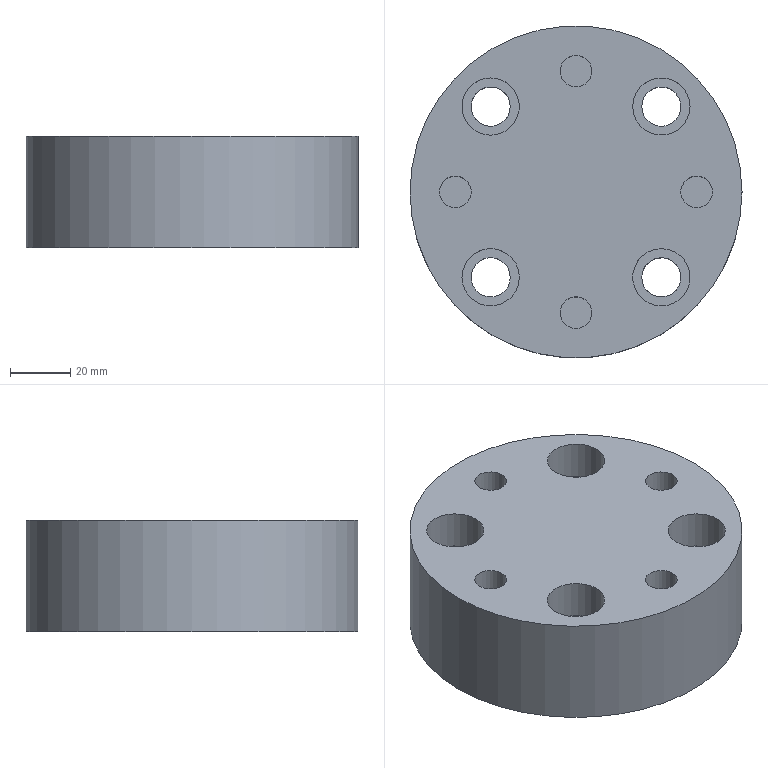NC program | NX | posted with a generic post | part box 110 x 110 x 37 mm
Whole program:
N10 G17 G21 G94 G90
(DRILLING , TOOL : ZXZ)
N12 T01 M6
N14 G54
N16 G17 G0 G90 X0. Y40. S3500 M3
N18 G43 Z30. H1
N20 G94 G81 G98 Z-1. F250. R3.
N22 X-28.284 Y28.284
N24 X-40. Y0.
N26 X-28.284 Y-28.284
N28 X0. Y-40.
N30 X28.284 Y-28.284
N32 X40. Y0.
N34 X28.284 Y28.284
N36 G80
N38 G0 X28.284 Y28.284 Z30.
N40 M5
(DRILLING_COPY , TOOL : 10.5ZT)
N42 T02 M6
N44 G54
N46 G17 G0 G90 X0. Y40. S1200 M3
N48 G43 Z30. H2
N50 G94 G83 G98 Z-28.155 F150. Q3. R3.
N52 X40. Y0.
N54 X0. Y-40.
N56 X-40. Y0.
N58 G80
N60 G0 X-40. Y0. Z30.
N62 M5
(DRILLING_COPY_COPY , TOOL : 13.0ZT)
N64 T03 M6
N66 G54
N68 G17 G0 G90 X-28.284 Y28.284 S500 M3
N70 G43 Z30. H3
N72 G94 G83 G98 Z-41.406 F150. Q3. R3.
N74 X28.284
N76 Y-28.284
N78 X-28.284
N80 G80
N82 G0 X-28.284 Y-28.284 Z30.
N84 M5
(HOLE_MILLING , TOOL : D10)
N86 T10 M6
N88 G54
N90 G17 G0 G90 X-28.284 Y28.284 S3000 M3
N92 G43 Z30. H10
N94 Z0.5
N96 G94 G3 X-26.034 Y26.034 R2.25 F2200.
N98 X-23.784 Y28.284 R2.25
N100 X-23.784 Y28.284 Z0.28 I-4.5 J0.
N102 X-23.784 Y28.284 Z0.06 I-4.5 J0.
N104 X-23.784 Y28.284 Z-0.16 I-4.5 J0.
N106 X-23.784 Y28.284 Z-0.38 I-4.5 J0.
N108 X-23.784 Y28.284 Z-0.6 I-4.5 J0.
N110 X-23.784 Y28.284 Z-0.82 I-4.5 J0.
N112 X-23.784 Y28.284 Z-1.04 I-4.5 J0.
N114 X-23.784 Y28.284 Z-1.26 I-4.5 J0.
N116 X-23.784 Y28.284 Z-1.48 I-4.5 J0.
N118 X-23.784 Y28.284 Z-1.7 I-4.5 J0.
N120 X-23.784 Y28.284 Z-1.92 I-4.5 J0.
N122 X-23.784 Y28.284 Z-2.14 I-4.5 J0.
N124 X-23.784 Y28.284 Z-2.36 I-4.5 J0.
N126 X-23.784 Y28.284 Z-2.58 I-4.5 J0.
N128 X-23.784 Y28.284 Z-2.8 I-4.5 J0.
N130 X-23.784 Y28.284 Z-3.02 I-4.5 J0.
N132 X-23.784 Y28.284 Z-3.24 I-4.5 J0.
N134 X-23.784 Y28.284 Z-3.46 I-4.5 J0.
N136 X-23.784 Y28.284 Z-3.68 I-4.5 J0.
N138 X-23.784 Y28.284 Z-3.9 I-4.5 J0.
N140 X-23.784 Y28.284 Z-4.12 I-4.5 J0.
N142 X-23.784 Y28.284 Z-4.34 I-4.5 J0.
N144 X-23.784 Y28.284 Z-4.56 I-4.5 J0.
N146 X-23.784 Y28.284 Z-4.78 I-4.5 J0.
N148 X-23.784 Y28.284 Z-5. I-4.5 J0.
N150 X-23.784 Y28.284 Z-5.22 I-4.5 J0.
N152 X-23.784 Y28.284 Z-5.44 I-4.5 J0.
N154 X-23.784 Y28.284 Z-5.66 I-4.5 J0.
N156 X-23.784 Y28.284 Z-5.88 I-4.5 J0.
N158 X-23.784 Y28.284 Z-6.1 I-4.5 J0.
N160 X-23.784 Y28.284 Z-6.32 I-4.5 J0.
N162 X-23.784 Y28.284 Z-6.54 I-4.5 J0.
N164 X-23.784 Y28.284 Z-6.76 I-4.5 J0.
N166 X-23.784 Y28.284 Z-6.98 I-4.5 J0.
N168 X-23.784 Y28.284 Z-7.2 I-4.5 J0.
N170 X-23.784 Y28.284 Z-7.42 I-4.5 J0.
N172 X-23.784 Y28.284 Z-7.64 I-4.5 J0.
N174 X-23.784 Y28.284 Z-7.86 I-4.5 J0.
N176 X-23.784 Y28.284 Z-8.08 I-4.5 J0.
N178 X-23.784 Y28.284 Z-8.3 I-4.5 J0.
N180 X-23.784 Y28.284 Z-8.52 I-4.5 J0.
N182 X-23.784 Y28.284 Z-8.74 I-4.5 J0.
N184 X-23.784 Y28.284 Z-8.96 I-4.5 J0.
N186 X-23.784 Y28.284 Z-9.18 I-4.5 J0.
N188 X-23.784 Y28.284 Z-9.4 I-4.5 J0.
N190 X-23.784 Y28.284 Z-9.62 I-4.5 J0.
N192 X-23.784 Y28.284 Z-9.84 I-4.5 J0.
N194 X-23.784 Y28.284 Z-10.06 I-4.5 J0.
N196 X-23.784 Y28.284 Z-10.28 I-4.5 J0.
N198 X-23.784 Y28.284 Z-10.5 I-4.5 J0.
N200 X-23.784 Y28.284 Z-10.72 I-4.5 J0.
N202 X-23.784 Y28.284 Z-10.94 I-4.5 J0.
N204 X-23.784 Y28.284 Z-11.16 I-4.5 J0.
N206 X-23.784 Y28.284 Z-11.38 I-4.5 J0.
N208 X-23.784 Y28.284 Z-11.6 I-4.5 J0.
N210 X-23.784 Y28.284 Z-11.82 I-4.5 J0.
N212 X-23.784 Y28.284 Z-12.04 I-4.5 J0.
N214 X-23.784 Y28.284 Z-12.26 I-4.5 J0.
N216 X-23.784 Y28.284 Z-12.48 I-4.5 J0.
N218 X-23.784 Y28.284 Z-12.7 I-4.5 J0.
N220 X-23.784 Y28.284 Z-12.92 I-4.5 J0.
N222 X-31.231 Y31.685 Z-13. R4.5
N224 X-31.685 Y25.337 R4.5
N226 X-31.231 Y31.685 R-4.5
N228 X-31.458 Y28.511 R2.25
N230 X-28.284 Y28.284 R2.25
N232 G0 Z30.
N234 X28.284
N236 Z0.5
N238 G3 X30.534 Y26.034 R2.25
N240 X32.784 Y28.284 R2.25
N242 X32.784 Y28.284 Z0.28 I-4.5 J0.
N244 X32.784 Y28.284 Z0.06 I-4.5 J0.
N246 X32.784 Y28.284 Z-0.16 I-4.5 J0.
N248 X32.784 Y28.284 Z-0.38 I-4.5 J0.
N250 X32.784 Y28.284 Z-0.6 I-4.5 J0.
N252 X32.784 Y28.284 Z-0.82 I-4.5 J0.
N254 X32.784 Y28.284 Z-1.04 I-4.5 J0.
N256 X32.784 Y28.284 Z-1.26 I-4.5 J0.
N258 X32.784 Y28.284 Z-1.48 I-4.5 J0.
N260 X32.784 Y28.284 Z-1.7 I-4.5 J0.
N262 X32.784 Y28.284 Z-1.92 I-4.5 J0.
N264 X32.784 Y28.284 Z-2.14 I-4.5 J0.
N266 X32.784 Y28.284 Z-2.36 I-4.5 J0.
N268 X32.784 Y28.284 Z-2.58 I-4.5 J0.
N270 X32.784 Y28.284 Z-2.8 I-4.5 J0.
N272 X32.784 Y28.284 Z-3.02 I-4.5 J0.
N274 X32.784 Y28.284 Z-3.24 I-4.5 J0.
N276 X32.784 Y28.284 Z-3.46 I-4.5 J0.
N278 X32.784 Y28.284 Z-3.68 I-4.5 J0.
N280 X32.784 Y28.284 Z-3.9 I-4.5 J0.
N282 X32.784 Y28.284 Z-4.12 I-4.5 J0.
N284 X32.784 Y28.284 Z-4.34 I-4.5 J0.
N286 X32.784 Y28.284 Z-4.56 I-4.5 J0.
N288 X32.784 Y28.284 Z-4.78 I-4.5 J0.
N290 X32.784 Y28.284 Z-5. I-4.5 J0.
N292 X32.784 Y28.284 Z-5.22 I-4.5 J0.
N294 X32.784 Y28.284 Z-5.44 I-4.5 J0.
N296 X32.784 Y28.284 Z-5.66 I-4.5 J0.
N298 X32.784 Y28.284 Z-5.88 I-4.5 J0.
N300 X32.784 Y28.284 Z-6.1 I-4.5 J0.
N302 X32.784 Y28.284 Z-6.32 I-4.5 J0.
N304 X32.784 Y28.284 Z-6.54 I-4.5 J0.
N306 X32.784 Y28.284 Z-6.76 I-4.5 J0.
N308 X32.784 Y28.284 Z-6.98 I-4.5 J0.
N310 X32.784 Y28.284 Z-7.2 I-4.5 J0.
N312 X32.784 Y28.284 Z-7.42 I-4.5 J0.
N314 X32.784 Y28.284 Z-7.64 I-4.5 J0.
N316 X32.784 Y28.284 Z-7.86 I-4.5 J0.
N318 X32.784 Y28.284 Z-8.08 I-4.5 J0.
N320 X32.784 Y28.284 Z-8.3 I-4.5 J0.
N322 X32.784 Y28.284 Z-8.52 I-4.5 J0.
N324 X32.784 Y28.284 Z-8.74 I-4.5 J0.
N326 X32.784 Y28.284 Z-8.96 I-4.5 J0.
N328 X32.784 Y28.284 Z-9.18 I-4.5 J0.
N330 X32.784 Y28.284 Z-9.4 I-4.5 J0.
N332 X32.784 Y28.284 Z-9.62 I-4.5 J0.
N334 X32.784 Y28.284 Z-9.84 I-4.5 J0.
N336 X32.784 Y28.284 Z-10.06 I-4.5 J0.
N338 X32.784 Y28.284 Z-10.28 I-4.5 J0.
N340 X32.784 Y28.284 Z-10.5 I-4.5 J0.
N342 X32.784 Y28.284 Z-10.72 I-4.5 J0.
N344 X32.784 Y28.284 Z-10.94 I-4.5 J0.
N346 X32.784 Y28.284 Z-11.16 I-4.5 J0.
N348 X32.784 Y28.284 Z-11.38 I-4.5 J0.
N350 X32.784 Y28.284 Z-11.6 I-4.5 J0.
N352 X32.784 Y28.284 Z-11.82 I-4.5 J0.
N354 X32.784 Y28.284 Z-12.04 I-4.5 J0.
N356 X32.784 Y28.284 Z-12.26 I-4.5 J0.
N358 X32.784 Y28.284 Z-12.48 I-4.5 J0.
N360 X32.784 Y28.284 Z-12.7 I-4.5 J0.
N362 X32.784 Y28.284 Z-12.92 I-4.5 J0.
N364 X25.337 Y31.685 Z-13. R4.5
N366 X24.883 Y25.337 R4.5
N368 X25.337 Y31.685 R-4.5
N370 X25.11 Y28.511 R2.25
N372 X28.284 Y28.284 R2.25
N374 G0 Z30.
N376 Y-28.284
N378 Z0.5
N380 G3 X30.534 Y-30.534 R2.25
N382 X32.784 Y-28.284 R2.25
N384 X32.784 Y-28.284 Z0.28 I-4.5 J0.
N386 X32.784 Y-28.284 Z0.06 I-4.5 J0.
N388 X32.784 Y-28.284 Z-0.16 I-4.5 J0.
N390 X32.784 Y-28.284 Z-0.38 I-4.5 J0.
N392 X32.784 Y-28.284 Z-0.6 I-4.5 J0.
N394 X32.784 Y-28.284 Z-0.82 I-4.5 J0.
N396 X32.784 Y-28.284 Z-1.04 I-4.5 J0.
N398 X32.784 Y-28.284 Z-1.26 I-4.5 J0.
N400 X32.784 Y-28.284 Z-1.48 I-4.5 J0.
N402 X32.784 Y-28.284 Z-1.7 I-4.5 J0.
N404 X32.784 Y-28.284 Z-1.92 I-4.5 J0.
N406 X32.784 Y-28.284 Z-2.14 I-4.5 J0.
N408 X32.784 Y-28.284 Z-2.36 I-4.5 J0.
N410 X32.784 Y-28.284 Z-2.58 I-4.5 J0.
N412 X32.784 Y-28.284 Z-2.8 I-4.5 J0.
N414 X32.784 Y-28.284 Z-3.02 I-4.5 J0.
N416 X32.784 Y-28.284 Z-3.24 I-4.5 J0.
N418 X32.784 Y-28.284 Z-3.46 I-4.5 J0.
N420 X32.784 Y-28.284 Z-3.68 I-4.5 J0.
N422 X32.784 Y-28.284 Z-3.9 I-4.5 J0.
N424 X32.784 Y-28.284 Z-4.12 I-4.5 J0.
N426 X32.784 Y-28.284 Z-4.34 I-4.5 J0.
N428 X32.784 Y-28.284 Z-4.56 I-4.5 J0.
N430 X32.784 Y-28.284 Z-4.78 I-4.5 J0.
N432 X32.784 Y-28.284 Z-5. I-4.5 J0.
N434 X32.784 Y-28.284 Z-5.22 I-4.5 J0.
N436 X32.784 Y-28.284 Z-5.44 I-4.5 J0.
N438 X32.784 Y-28.284 Z-5.66 I-4.5 J0.
N440 X32.784 Y-28.284 Z-5.88 I-4.5 J0.
N442 X32.784 Y-28.284 Z-6.1 I-4.5 J0.
N444 X32.784 Y-28.284 Z-6.32 I-4.5 J0.
N446 X32.784 Y-28.284 Z-6.54 I-4.5 J0.
N448 X32.784 Y-28.284 Z-6.76 I-4.5 J0.
N450 X32.784 Y-28.284 Z-6.98 I-4.5 J0.
N452 X32.784 Y-28.284 Z-7.2 I-4.5 J0.
N454 X32.784 Y-28.284 Z-7.42 I-4.5 J0.
N456 X32.784 Y-28.284 Z-7.64 I-4.5 J0.
N458 X32.784 Y-28.284 Z-7.86 I-4.5 J0.
N460 X32.784 Y-28.284 Z-8.08 I-4.5 J0.
N462 X32.784 Y-28.284 Z-8.3 I-4.5 J0.
N464 X32.784 Y-28.284 Z-8.52 I-4.5 J0.
N466 X32.784 Y-28.284 Z-8.74 I-4.5 J0.
N468 X32.784 Y-28.284 Z-8.96 I-4.5 J0.
N470 X32.784 Y-28.284 Z-9.18 I-4.5 J0.
N472 X32.784 Y-28.284 Z-9.4 I-4.5 J0.
N474 X32.784 Y-28.284 Z-9.62 I-4.5 J0.
N476 X32.784 Y-28.284 Z-9.84 I-4.5 J0.
N478 X32.784 Y-28.284 Z-10.06 I-4.5 J0.
N480 X32.784 Y-28.284 Z-10.28 I-4.5 J0.
N482 X32.784 Y-28.284 Z-10.5 I-4.5 J0.
N484 X32.784 Y-28.284 Z-10.72 I-4.5 J0.
N486 X32.784 Y-28.284 Z-10.94 I-4.5 J0.
N488 X32.784 Y-28.284 Z-11.16 I-4.5 J0.
N490 X32.784 Y-28.284 Z-11.38 I-4.5 J0.
N492 X32.784 Y-28.284 Z-11.6 I-4.5 J0.
N494 X32.784 Y-28.284 Z-11.82 I-4.5 J0.
N496 X32.784 Y-28.284 Z-12.04 I-4.5 J0.
N498 X32.784 Y-28.284 Z-12.26 I-4.5 J0.
N500 X32.784 Y-28.284 Z-12.48 I-4.5 J0.
N502 X32.784 Y-28.284 Z-12.7 I-4.5 J0.
N504 X32.784 Y-28.284 Z-12.92 I-4.5 J0.
N506 X25.337 Y-24.883 Z-13. R4.5
N508 X24.883 Y-31.231 R4.5
N510 X25.337 Y-24.883 R-4.5
N512 X25.11 Y-28.057 R2.25
N514 X28.284 Y-28.284 R2.25
N516 G0 Z30.
N518 X-28.284
N520 Z0.5
N522 G3 X-26.034 Y-30.534 R2.25
N524 X-23.784 Y-28.284 R2.25
N526 X-23.784 Y-28.284 Z0.28 I-4.5 J0.
N528 X-23.784 Y-28.284 Z0.06 I-4.5 J0.
N530 X-23.784 Y-28.284 Z-0.16 I-4.5 J0.
N532 X-23.784 Y-28.284 Z-0.38 I-4.5 J0.
N534 X-23.784 Y-28.284 Z-0.6 I-4.5 J0.
N536 X-23.784 Y-28.284 Z-0.82 I-4.5 J0.
N538 X-23.784 Y-28.284 Z-1.04 I-4.5 J0.
N540 X-23.784 Y-28.284 Z-1.26 I-4.5 J0.
N542 X-23.784 Y-28.284 Z-1.48 I-4.5 J0.
N544 X-23.784 Y-28.284 Z-1.7 I-4.5 J0.
N546 X-23.784 Y-28.284 Z-1.92 I-4.5 J0.
N548 X-23.784 Y-28.284 Z-2.14 I-4.5 J0.
N550 X-23.784 Y-28.284 Z-2.36 I-4.5 J0.
N552 X-23.784 Y-28.284 Z-2.58 I-4.5 J0.
N554 X-23.784 Y-28.284 Z-2.8 I-4.5 J0.
N556 X-23.784 Y-28.284 Z-3.02 I-4.5 J0.
N558 X-23.784 Y-28.284 Z-3.24 I-4.5 J0.
N560 X-23.784 Y-28.284 Z-3.46 I-4.5 J0.
N562 X-23.784 Y-28.284 Z-3.68 I-4.5 J0.
N564 X-23.784 Y-28.284 Z-3.9 I-4.5 J0.
N566 X-23.784 Y-28.284 Z-4.12 I-4.5 J0.
N568 X-23.784 Y-28.284 Z-4.34 I-4.5 J0.
N570 X-23.784 Y-28.284 Z-4.56 I-4.5 J0.
N572 X-23.784 Y-28.284 Z-4.78 I-4.5 J0.
N574 X-23.784 Y-28.284 Z-5. I-4.5 J0.
N576 X-23.784 Y-28.284 Z-5.22 I-4.5 J0.
N578 X-23.784 Y-28.284 Z-5.44 I-4.5 J0.
N580 X-23.784 Y-28.284 Z-5.66 I-4.5 J0.
N582 X-23.784 Y-28.284 Z-5.88 I-4.5 J0.
N584 X-23.784 Y-28.284 Z-6.1 I-4.5 J0.
N586 X-23.784 Y-28.284 Z-6.32 I-4.5 J0.
N588 X-23.784 Y-28.284 Z-6.54 I-4.5 J0.
N590 X-23.784 Y-28.284 Z-6.76 I-4.5 J0.
N592 X-23.784 Y-28.284 Z-6.98 I-4.5 J0.
N594 X-23.784 Y-28.284 Z-7.2 I-4.5 J0.
N596 X-23.784 Y-28.284 Z-7.42 I-4.5 J0.
N598 X-23.784 Y-28.284 Z-7.64 I-4.5 J0.
N600 X-23.784 Y-28.284 Z-7.86 I-4.5 J0.
N602 X-23.784 Y-28.284 Z-8.08 I-4.5 J0.
N604 X-23.784 Y-28.284 Z-8.3 I-4.5 J0.
N606 X-23.784 Y-28.284 Z-8.52 I-4.5 J0.
N608 X-23.784 Y-28.284 Z-8.74 I-4.5 J0.
N610 X-23.784 Y-28.284 Z-8.96 I-4.5 J0.
N612 X-23.784 Y-28.284 Z-9.18 I-4.5 J0.
N614 X-23.784 Y-28.284 Z-9.4 I-4.5 J0.
N616 X-23.784 Y-28.284 Z-9.62 I-4.5 J0.
N618 X-23.784 Y-28.284 Z-9.84 I-4.5 J0.
N620 X-23.784 Y-28.284 Z-10.06 I-4.5 J0.
N622 X-23.784 Y-28.284 Z-10.28 I-4.5 J0.
N624 X-23.784 Y-28.284 Z-10.5 I-4.5 J0.
N626 X-23.784 Y-28.284 Z-10.72 I-4.5 J0.
N628 X-23.784 Y-28.284 Z-10.94 I-4.5 J0.
N630 X-23.784 Y-28.284 Z-11.16 I-4.5 J0.
N632 X-23.784 Y-28.284 Z-11.38 I-4.5 J0.
N634 X-23.784 Y-28.284 Z-11.6 I-4.5 J0.
N636 X-23.784 Y-28.284 Z-11.82 I-4.5 J0.
N638 X-23.784 Y-28.284 Z-12.04 I-4.5 J0.
N640 X-23.784 Y-28.284 Z-12.26 I-4.5 J0.
N642 X-23.784 Y-28.284 Z-12.48 I-4.5 J0.
N644 X-23.784 Y-28.284 Z-12.7 I-4.5 J0.
N646 X-23.784 Y-28.284 Z-12.92 I-4.5 J0.
N648 X-31.231 Y-24.883 Z-13. R4.5
N650 X-31.685 Y-31.231 R4.5
N652 X-31.231 Y-24.883 R-4.5
N654 X-31.458 Y-28.057 R2.25
N656 X-28.284 Y-28.284 R2.25
N658 G0 Z30.
N660 M5
(PLANAR_MILL , TOOL : D6A45)
N662 T07 M6
N664 G54
N666 G17 G0 G90 X21.065 Y29.909 S7500 M3
N668 G43 Z30. H7
N670 Z2.
N672 G94 G1 Z-1. F1250.
N674 X20.041 Y29.05
N676 G3 X19.684 Y28.284 R1.
N678 X28.284 Y19.684 R8.6
N680 X19.684 Y28.284 R-8.6
N682 X20.041 Y27.518 R1.
N684 G1 X21.065 Y26.66
N686 Z2.
N688 G0 Z30.
N690 X-3.094 Y40.594
N692 Z2.
N694 G1 Z-1.
N696 X-3.993 Y40.766
N698 G3 X-4.35 Y40. R1.
N700 X0. Y35.65 R4.35
N702 X-4.35 Y40. R-4.35
N704 X-3.993 Y39.234 R1.
N706 G1 X-3.094 Y39.406
N708 Z2.
N710 G0 Z30.
N712 X-35.504 Y29.909
N714 Z2.
N716 G1 Z-1.
N718 X-36.527 Y29.05
N720 G3 X-36.884 Y28.284 R1.
N722 X-28.284 Y19.684 R8.6
N724 X-36.884 Y28.284 R-8.6
N726 X-36.527 Y27.518 R1.
N728 G1 X-35.504 Y26.66
N730 Z2.
N732 G0 Z30.
N734 X-43.094 Y0.594
N736 Z2.
N738 G1 Z-1.
N740 X-43.993 Y0.766
N742 G3 X-44.35 Y0. R1.
N744 X-40. Y-4.35 R4.35
N746 X-44.35 Y0. R-4.35
N748 X-43.993 Y-0.766 R1.
N750 G1 X-43.094 Y-0.594
N752 Z2.
N754 G0 Z30.
N756 X-21.065 Y-29.909
N758 Z2.
N760 G1 Z-1.
N762 X-20.041 Y-29.05
N764 G3 X-19.684 Y-28.284 R1.
N766 X-28.284 Y-19.684 R8.6
N768 X-19.684 Y-28.284 R-8.6
N770 X-20.041 Y-27.518 R1.
N772 G1 X-21.065 Y-26.66
N774 Z2.
N776 G0 Z30.
N778 X-3.094 Y-39.406
N780 Z2.
N782 G1 Z-1.
N784 X-3.993 Y-39.234
N786 G3 X-4.35 Y-40. R1.
N788 X0. Y-44.35 R4.35
N790 X-4.35 Y-40. R-4.35
N792 X-3.993 Y-40.766 R1.
N794 G1 X-3.094 Y-40.594
N796 Z2.
N798 G0 Z30.
N800 X21.065 Y-26.66
N802 Z2.
N804 G1 Z-1.
N806 X20.041 Y-27.518
N808 G3 X19.684 Y-28.284 R1.
N810 X28.284 Y-36.884 R8.6
N812 X19.684 Y-28.284 R-8.6
N814 X20.041 Y-29.05 R1.
N816 G1 X21.065 Y-29.909
N818 Z2.
N820 G0 Z30.
N822 X36.906 Y0.594
N824 Z2.
N826 G1 Z-1.
N828 X36.007 Y0.766
N830 G3 X35.65 Y0. R1.
N832 X40. Y-4.35 R4.35
N834 X35.65 Y0. R-4.35
N836 X36.007 Y-0.766 R1.
N838 G1 X36.906 Y-0.594
N840 Z2.
N842 G0 Z30.
N844 M5
N846 M2